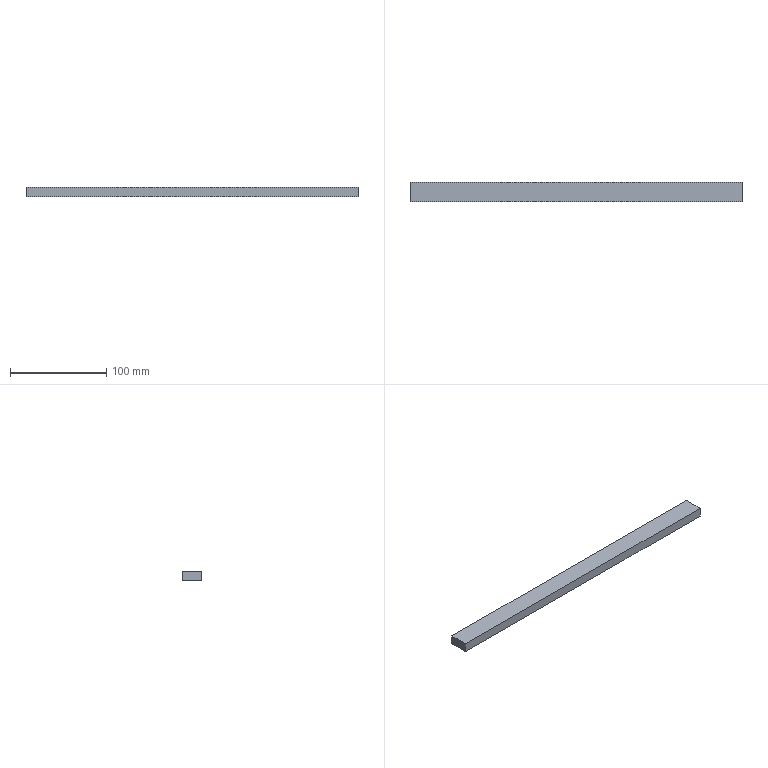Part | SolidWorks | features Extrusion 1 | 1 solid | 6 faces | box 345 x 20 x 10 mm | volume 69000 mm3 | plane 6
STEP:
#1=CARTESIAN_POINT('',(172.5,-10.,0.));
#2=VERTEX_POINT('',#1);
#3=CARTESIAN_POINT('',(172.5,10.,0.));
#4=VERTEX_POINT('',#3);
#5=CARTESIAN_POINT('',(172.5,10.,0.));
#6=DIRECTION('',(0.,1.,0.));
#7=VECTOR('',#6,1000.);
#8=LINE('',#5,#7);
#9=EDGE_CURVE('',#2,#4,#8,.T.);
#10=ORIENTED_EDGE('',*,*,#9,.T.);
#11=CARTESIAN_POINT('',(172.5,10.,10.));
#12=VERTEX_POINT('',#11);
#13=CARTESIAN_POINT('',(172.5,10.,10.));
#14=DIRECTION('',(0.,0.,-1.));
#15=VECTOR('',#14,1000.);
#16=LINE('',#13,#15);
#17=EDGE_CURVE('',#12,#4,#16,.T.);
#18=ORIENTED_EDGE('',*,*,#17,.F.);
#19=CARTESIAN_POINT('',(172.5,-10.,10.));
#20=VERTEX_POINT('',#19);
#21=CARTESIAN_POINT('',(172.5,10.,10.));
#22=DIRECTION('',(0.,1.,0.));
#23=VECTOR('',#22,1000.);
#24=LINE('',#21,#23);
#25=EDGE_CURVE('',#20,#12,#24,.T.);
#26=ORIENTED_EDGE('',*,*,#25,.F.);
#27=CARTESIAN_POINT('',(172.5,-10.,10.));
#28=DIRECTION('',(0.,0.,-1.));
#29=VECTOR('',#28,1000.);
#30=LINE('',#27,#29);
#31=EDGE_CURVE('',#20,#2,#30,.T.);
#32=ORIENTED_EDGE('',*,*,#31,.T.);
#33=EDGE_LOOP('',(#10,#18,#26,#32));
#34=FACE_OUTER_BOUND('',#33,.T.);
#35=CARTESIAN_POINT('',(172.5,10.,10.));
#36=DIRECTION('',(-1.,0.,0.));
#37=DIRECTION('',(0.,0.,1.));
#38=AXIS2_PLACEMENT_3D('',#35,#36,#37);
#39=PLANE('',#38);
#40=ADVANCED_FACE('',(#34),#39,.F.);
#41=CARTESIAN_POINT('',(-172.5,10.,0.));
#42=VERTEX_POINT('',#41);
#43=CARTESIAN_POINT('',(-172.5,10.,0.));
#44=DIRECTION('',(-1.,0.,0.));
#45=VECTOR('',#44,1000.);
#46=LINE('',#43,#45);
#47=EDGE_CURVE('',#4,#42,#46,.T.);
#48=ORIENTED_EDGE('',*,*,#47,.T.);
#49=CARTESIAN_POINT('',(-172.5,10.,10.));
#50=VERTEX_POINT('',#49);
#51=CARTESIAN_POINT('',(-172.5,10.,10.));
#52=DIRECTION('',(0.,0.,-1.));
#53=VECTOR('',#52,1000.);
#54=LINE('',#51,#53);
#55=EDGE_CURVE('',#50,#42,#54,.T.);
#56=ORIENTED_EDGE('',*,*,#55,.F.);
#57=CARTESIAN_POINT('',(-172.5,10.,10.));
#58=DIRECTION('',(-1.,0.,0.));
#59=VECTOR('',#58,1000.);
#60=LINE('',#57,#59);
#61=EDGE_CURVE('',#12,#50,#60,.T.);
#62=ORIENTED_EDGE('',*,*,#61,.F.);
#63=ORIENTED_EDGE('',*,*,#17,.T.);
#64=EDGE_LOOP('',(#48,#56,#62,#63));
#65=FACE_OUTER_BOUND('',#64,.T.);
#66=CARTESIAN_POINT('',(-172.5,10.,10.));
#67=DIRECTION('',(0.,-1.,0.));
#68=DIRECTION('',(0.,0.,-1.));
#69=AXIS2_PLACEMENT_3D('',#66,#67,#68);
#70=PLANE('',#69);
#71=ADVANCED_FACE('',(#65),#70,.F.);
#72=CARTESIAN_POINT('',(-172.5,-10.,0.));
#73=VERTEX_POINT('',#72);
#74=CARTESIAN_POINT('',(-172.5,10.,0.));
#75=DIRECTION('',(0.,-1.,0.));
#76=VECTOR('',#75,1000.);
#77=LINE('',#74,#76);
#78=EDGE_CURVE('',#42,#73,#77,.T.);
#79=ORIENTED_EDGE('',*,*,#78,.T.);
#80=CARTESIAN_POINT('',(-172.5,-10.,10.));
#81=VERTEX_POINT('',#80);
#82=CARTESIAN_POINT('',(-172.5,-10.,10.));
#83=DIRECTION('',(0.,0.,-1.));
#84=VECTOR('',#83,1000.);
#85=LINE('',#82,#84);
#86=EDGE_CURVE('',#81,#73,#85,.T.);
#87=ORIENTED_EDGE('',*,*,#86,.F.);
#88=CARTESIAN_POINT('',(-172.5,10.,10.));
#89=DIRECTION('',(0.,-1.,0.));
#90=VECTOR('',#89,1000.);
#91=LINE('',#88,#90);
#92=EDGE_CURVE('',#50,#81,#91,.T.);
#93=ORIENTED_EDGE('',*,*,#92,.F.);
#94=ORIENTED_EDGE('',*,*,#55,.T.);
#95=EDGE_LOOP('',(#79,#87,#93,#94));
#96=FACE_OUTER_BOUND('',#95,.T.);
#97=CARTESIAN_POINT('',(-172.5,10.,10.));
#98=DIRECTION('',(1.,0.,0.));
#99=DIRECTION('',(0.,0.,-1.));
#100=AXIS2_PLACEMENT_3D('',#97,#98,#99);
#101=PLANE('',#100);
#102=ADVANCED_FACE('',(#96),#101,.F.);
#103=CARTESIAN_POINT('',(-172.5,-10.,0.));
#104=DIRECTION('',(1.,0.,0.));
#105=VECTOR('',#104,1000.);
#106=LINE('',#103,#105);
#107=EDGE_CURVE('',#73,#2,#106,.T.);
#108=ORIENTED_EDGE('',*,*,#107,.T.);
#109=ORIENTED_EDGE('',*,*,#31,.F.);
#110=CARTESIAN_POINT('',(-172.5,-10.,10.));
#111=DIRECTION('',(1.,0.,0.));
#112=VECTOR('',#111,1000.);
#113=LINE('',#110,#112);
#114=EDGE_CURVE('',#81,#20,#113,.T.);
#115=ORIENTED_EDGE('',*,*,#114,.F.);
#116=ORIENTED_EDGE('',*,*,#86,.T.);
#117=EDGE_LOOP('',(#108,#109,#115,#116));
#118=FACE_OUTER_BOUND('',#117,.T.);
#119=CARTESIAN_POINT('',(-172.5,-10.,10.));
#120=DIRECTION('',(0.,1.,0.));
#121=DIRECTION('',(0.,0.,1.));
#122=AXIS2_PLACEMENT_3D('',#119,#120,#121);
#123=PLANE('',#122);
#124=ADVANCED_FACE('',(#118),#123,.F.);
#125=ORIENTED_EDGE('',*,*,#25,.T.);
#126=ORIENTED_EDGE('',*,*,#61,.T.);
#127=ORIENTED_EDGE('',*,*,#92,.T.);
#128=ORIENTED_EDGE('',*,*,#114,.T.);
#129=EDGE_LOOP('',(#125,#126,#127,#128));
#130=FACE_OUTER_BOUND('',#129,.T.);
#131=CARTESIAN_POINT('',(0.,0.,10.));
#132=DIRECTION('',(0.,0.,1.));
#133=DIRECTION('',(1.,0.,0.));
#134=AXIS2_PLACEMENT_3D('',#131,#132,#133);
#135=PLANE('',#134);
#136=ADVANCED_FACE('',(#130),#135,.T.);
#137=ORIENTED_EDGE('',*,*,#9,.F.);
#138=ORIENTED_EDGE('',*,*,#107,.F.);
#139=ORIENTED_EDGE('',*,*,#78,.F.);
#140=ORIENTED_EDGE('',*,*,#47,.F.);
#141=EDGE_LOOP('',(#137,#138,#139,#140));
#142=FACE_OUTER_BOUND('',#141,.T.);
#143=CARTESIAN_POINT('',(0.,0.,0.));
#144=DIRECTION('',(0.,0.,1.));
#145=DIRECTION('',(1.,0.,0.));
#146=AXIS2_PLACEMENT_3D('',#143,#144,#145);
#147=PLANE('',#146);
#148=ADVANCED_FACE('',(#142),#147,.F.);
#149=CLOSED_SHELL('',(#40,#71,#102,#124,#136,#148));
#150=MANIFOLD_SOLID_BREP('',#149);
#151=CARTESIAN_POINT('',(0.,0.,0.));
#152=DIRECTION('',(0.,0.,1.));
#153=DIRECTION('',(1.,0.,0.));
#154=AXIS2_PLACEMENT_3D('',#151,#152,#153);
#155=(LENGTH_UNIT()NAMED_UNIT(*)SI_UNIT(.MILLI.,.METRE.));
#156=UNCERTAINTY_MEASURE_WITH_UNIT(LENGTH_MEASURE(0.00001),#155,'','');
#157=(NAMED_UNIT(*)PLANE_ANGLE_UNIT()SI_UNIT($,.RADIAN.));
#158=(NAMED_UNIT(*)SI_UNIT($,.STERADIAN.)SOLID_ANGLE_UNIT());
#159=(GEOMETRIC_REPRESENTATION_CONTEXT(3)GLOBAL_UNCERTAINTY_ASSIGNED_CONTEXT((#156))GLOBAL_UNIT_ASSIGNED_CONTEXT((#155,#157,#158))REPRESENTATION_CONTEXT('',''));
#160=ADVANCED_BREP_SHAPE_REPRESENTATION('',(#150,#154),#159);